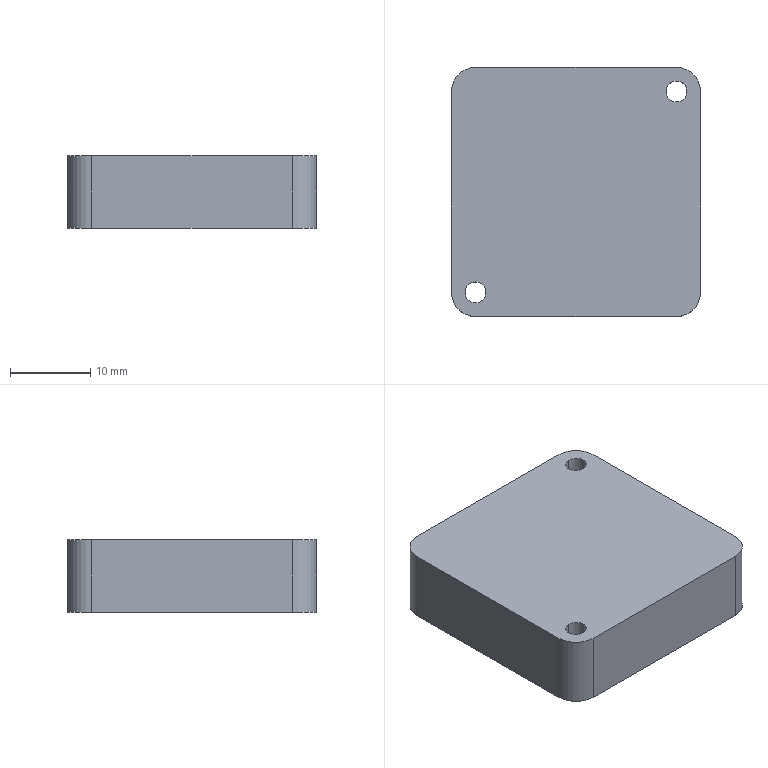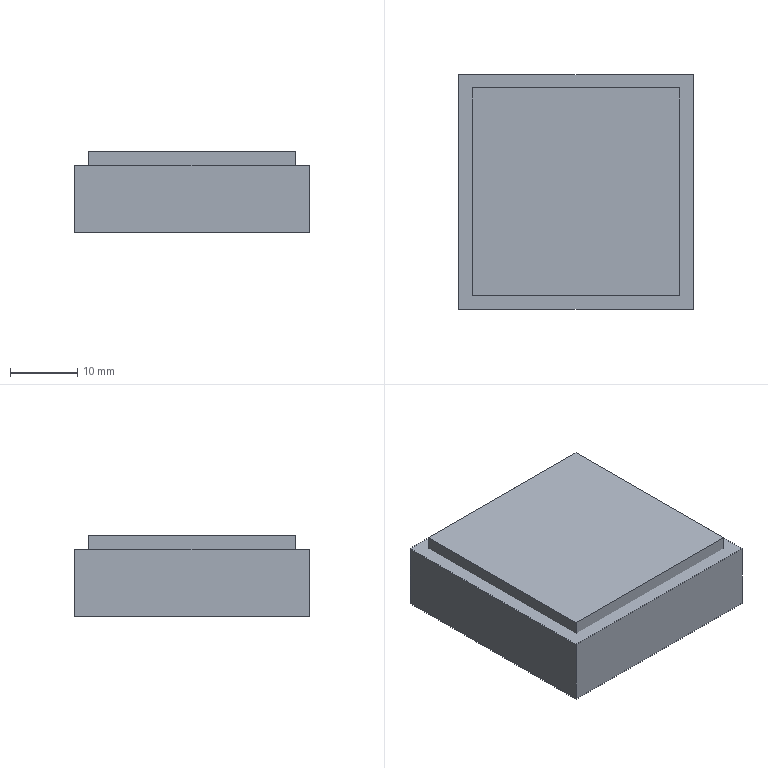CAM job | NX | 3-axis milling, drilling | part box 31 x 31 x 9 mm | stock box 35 x 35 x 12 mm
Tools:
number,name,description,diameter,corner_radius,flute_length,length,flutes
1,D63,Milling Tool-5 Parameters,63.0,0.0,50.0,75.0,2
7,D6A45,Milling Tool-5 Parameters,6.0,0.0,50.0,75.0,2
12,2.6ZT,Drilling Tool,2.6,0.0,35.0,50.0,2
13,M3,Milling Tool-5 Parameters,2.6,0.0,50.0,75.0,2
10,D10,Milling Tool-5 Parameters,10.0,0.0,50.0,75.0,2
Operations:
program,operation,operation_type,tool,method,geometry_group,spindle_rpm,surface_speed,feed_per_tooth,feed_cut,feed_plunge,cut_length_mm,path_length_mm,cut_time_min,machine_time_min
1,FLOOR_WALL,VolumeBased25DMillingOperation,D63,METHOD,A,6500.0,1286.0,0.0962,1250.0,100.0,110.0,164.0,0.088,0.0934
1,DRILLING,Operation,D6A45,METHOD,A,5000.0,94.0,0.025,250.0,0.0,9.2,116.882,0.0368,0.0476
1,DRILLING_COPY,Operation,2.6ZT,METHOD,A,2000.0,16.0,0.03,120.0,0.0,28.562,155.607,0.238,0.2507
1,DRILLING_COPY_COPY,Operation,M3,METHOD,A,300.0,2.0,0.0008,0.5,0.0,25.0,148.482,50.0,50.012
1,ZLEVEL_PROFILE,ZLevelMilling,D10,METHOD,A,9500.0,298.0,0.1316,2500.0,1000.0,1464.663,1530.663,0.6145,0.6211
1,ZLEVEL_PROFILE_COPY,ZLevelMilling,D10,METHOD,A,9500.0,298.0,0.0632,1200.0,1000.0,158.665,233.665,0.1329,0.1404
1,PLANAR_MILL,PlanarMilling,D6A45,METHOD,A,9500.0,179.0,0.0658,1250.0,100.0,141.149,363.855,0.1129,0.1352
2,FLOOR_WALL_COPY,VolumeBased25DMillingOperation,D63,METHOD,B,6500.0,1286.0,0.0962,1250.0,100.0,318.0,674.001,0.2544,0.29
2,PLANAR_MILL_COPY,PlanarMilling,D6A45,METHOD,B,9500.0,179.0,0.0658,1250.0,100.0,141.149,364.437,0.1129,0.1352